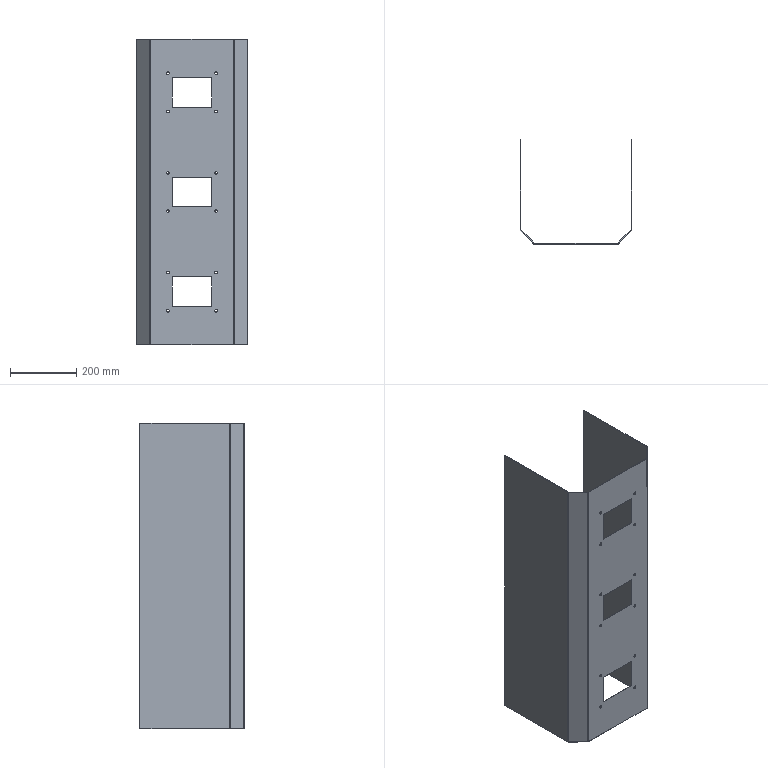Part | SolidWorks | features MirrorPattern 2, FlatPattern 1, ICE 1, SMBaseFlange 1, SheetMetal 1 | 1 solid | 74 faces | box 337 x 313.5 x 920 mm | volume 1609120 mm3 | plane 42 | cylinder 32 | commonest cylinder face diameters 8 x24 1.473 x4 5.473 x4